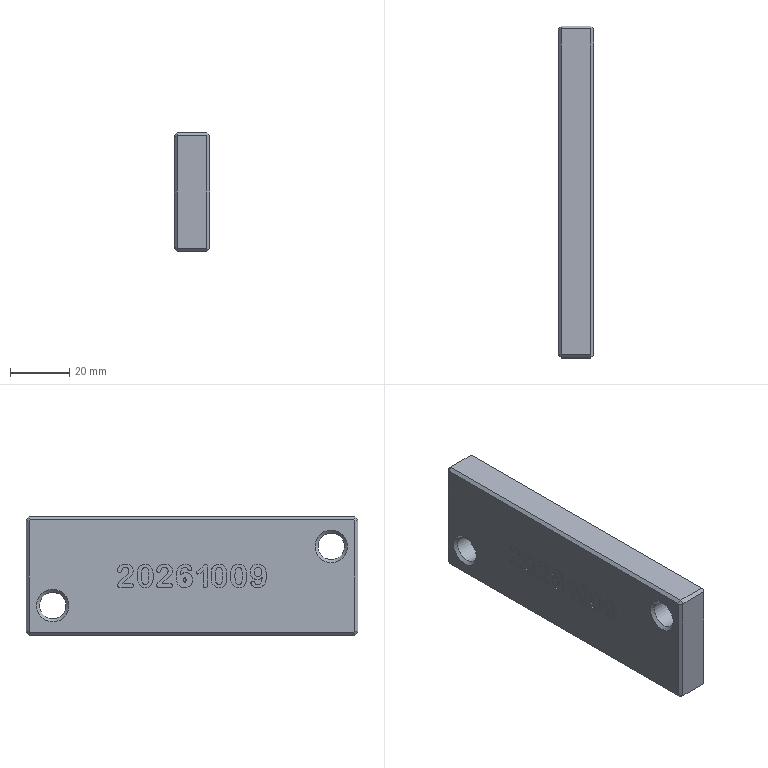Part | NX | features BREP 8, CHAMFER 2, solid 2, SUBTRACT 1 | 1 solid | 85 faces | box 12 x 112 x 40 mm | volume 51813 mm3 | spline 44 | plane 35 | cone 4 | cylinder 2 | commonest cylinder face diameters 9 x2